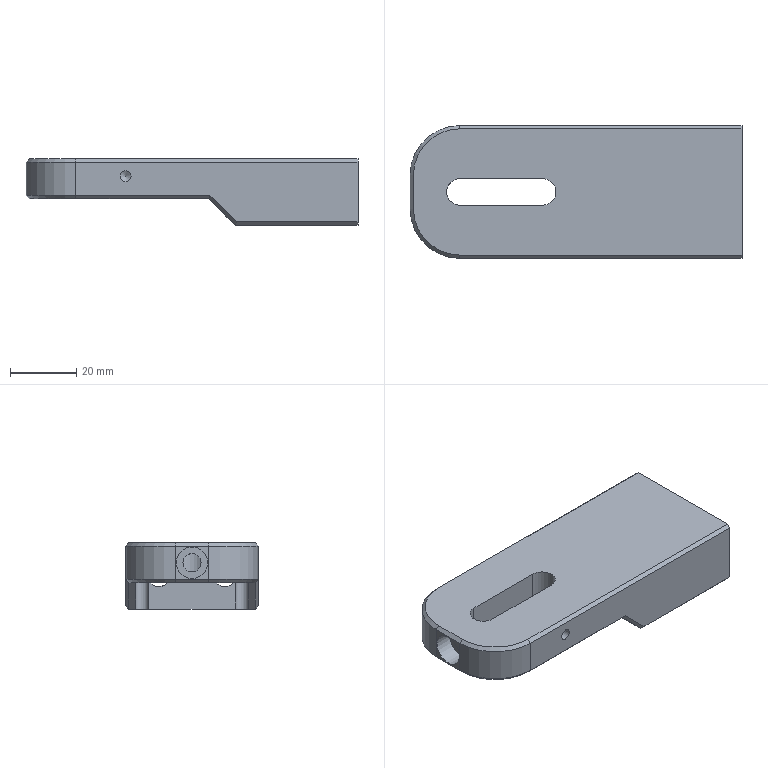Part | 1 solid | 48 faces | box 100 x 40 x 20 mm | volume 33187 mm3 | plane 28 | cylinder 14 | cone 6 | commonest cylinder face diameters 4 x4 3.3 x2 6.5 x2 8 x2 30 x2 5.5 x1
STEP:
#1=CARTESIAN_POINT('',(-37.905,2.75,-6.));
#2=VERTEX_POINT('',#1);
#3=CARTESIAN_POINT('',(-38.064,2.588,-4.884));
#4=CARTESIAN_POINT('',(-37.826,2.83,-6.002));
#5=CARTESIAN_POINT('',(-38.062,2.593,-7.11));
#6=CARTESIAN_POINT('',(-38.499,2.,-7.979));
#7=CARTESIAN_POINT('',(-38.885,1.129,-8.588));
#8=CARTESIAN_POINT('',(-39.115,-0.3754,-8.911));
#9=CARTESIAN_POINT('',(-38.65,-1.807,-8.274));
#10=CARTESIAN_POINT('',(-38.065,-2.587,-7.117));
#11=CARTESIAN_POINT('',(-37.826,-2.83,-6.007));
#12=CARTESIAN_POINT('',(-38.061,-2.591,-4.891));
#13=CARTESIAN_POINT('',(-38.645,-1.817,-3.733));
#14=CARTESIAN_POINT('',(-39.236,-0.009899,-2.929));
#15=CARTESIAN_POINT('',(-38.648,1.814,-3.73));
#16=CARTESIAN_POINT('',(-38.064,2.588,-4.884));
#17=CARTESIAN_POINT('',(-37.826,2.83,-6.002));
#18=CARTESIAN_POINT('',(-38.062,2.593,-7.11));
#19=B_SPLINE_CURVE_WITH_KNOTS('',3,(#3,#4,#5,#6,#7,#8,#9,#10,#11,#12,#13,#14,#15,#16,#17,#18),.UNSPECIFIED.,.T.,.F.,(1,1,1,1,1,1,1,1,1,1,1,1,1,1,1,1,1,1,1,1),(-0.004449,-0.002224,-0.001112,0.,0.001112,0.002224,0.003337,0.004449,0.006673,0.007786,0.008898,0.01001,0.01112,0.01335,0.01557,0.01668,0.0178,0.01891,0.02002,0.02113),.UNSPECIFIED.);
#20=EDGE_CURVE('',#2,#2,#19,.T.);
#21=ORIENTED_EDGE('',*,*,#20,.F.);
#22=EDGE_LOOP('',(#21));
#23=FACE_BOUND('',#22,.T.);
#24=CARTESIAN_POINT('',(-44.5,2.75,-6.));
#25=VERTEX_POINT('',#24);
#26=CARTESIAN_POINT('',(-44.5,0.,-6.));
#27=DIRECTION('',(1.,0.,0.));
#28=DIRECTION('',(0.,1.,0.));
#29=AXIS2_PLACEMENT_3D('',#26,#27,#28);
#30=CIRCLE('',#29,2.75);
#31=EDGE_CURVE('',#25,#25,#30,.T.);
#32=ORIENTED_EDGE('',*,*,#31,.F.);
#33=EDGE_LOOP('',(#32));
#34=FACE_BOUND('',#33,.T.);
#35=CARTESIAN_POINT('',(-35.,0.,-6.));
#36=DIRECTION('',(-1.,0.,0.));
#37=DIRECTION('',(0.,-1.,0.));
#38=AXIS2_PLACEMENT_3D('',#35,#36,#37);
#39=CYLINDRICAL_SURFACE('',#38,2.75);
#40=ADVANCED_FACE('',(#23,#34),#39,.F.);
#41=CARTESIAN_POINT('',(-50.,4.75,-6.));
#42=VERTEX_POINT('',#41);
#43=CARTESIAN_POINT('',(-50.,0.,-6.));
#44=DIRECTION('',(-1.,0.,0.));
#45=DIRECTION('',(0.,1.,0.));
#46=AXIS2_PLACEMENT_3D('',#43,#44,#45);
#47=CIRCLE('',#46,4.75);
#48=EDGE_CURVE('',#42,#42,#47,.T.);
#49=ORIENTED_EDGE('',*,*,#48,.F.);
#50=EDGE_LOOP('',(#49));
#51=FACE_BOUND('',#50,.T.);
#52=CARTESIAN_POINT('',(-50.,5.,-1.));
#53=VERTEX_POINT('',#52);
#54=CARTESIAN_POINT('',(-50.,5.,-11.));
#55=VERTEX_POINT('',#54);
#56=CARTESIAN_POINT('',(-50.,5.,-20.));
#57=DIRECTION('',(0.,0.,-1.));
#58=VECTOR('',#57,1000.);
#59=LINE('',#56,#58);
#60=EDGE_CURVE('',#53,#55,#59,.T.);
#61=ORIENTED_EDGE('',*,*,#60,.T.);
#62=CARTESIAN_POINT('',(-50.,-5.,-11.));
#63=VERTEX_POINT('',#62);
#64=CARTESIAN_POINT('',(-50.,-20.,-11.));
#65=DIRECTION('',(0.,-1.,0.));
#66=VECTOR('',#65,1000.);
#67=LINE('',#64,#66);
#68=EDGE_CURVE('',#55,#63,#67,.T.);
#69=ORIENTED_EDGE('',*,*,#68,.T.);
#70=CARTESIAN_POINT('',(-50.,-5.,-1.));
#71=VERTEX_POINT('',#70);
#72=CARTESIAN_POINT('',(-50.,-5.,-20.));
#73=DIRECTION('',(0.,0.,1.));
#74=VECTOR('',#73,1000.);
#75=LINE('',#72,#74);
#76=EDGE_CURVE('',#63,#71,#75,.T.);
#77=ORIENTED_EDGE('',*,*,#76,.T.);
#78=CARTESIAN_POINT('',(-50.,-20.,-1.));
#79=DIRECTION('',(0.,1.,0.));
#80=VECTOR('',#79,1000.);
#81=LINE('',#78,#80);
#82=EDGE_CURVE('',#71,#53,#81,.T.);
#83=ORIENTED_EDGE('',*,*,#82,.T.);
#84=EDGE_LOOP('',(#61,#69,#77,#83));
#85=FACE_BOUND('',#84,.T.);
#86=CARTESIAN_POINT('',(-50.,-20.,-20.));
#87=DIRECTION('',(1.,0.,0.));
#88=DIRECTION('',(0.,1.,0.));
#89=AXIS2_PLACEMENT_3D('',#86,#87,#88);
#90=PLANE('',#89);
#91=ADVANCED_FACE('',(#51,#85),#90,.F.);
#92=CARTESIAN_POINT('',(-18.35,20.,-5.25));
#93=VERTEX_POINT('',#92);
#94=CARTESIAN_POINT('',(-20.,20.,-5.25));
#95=DIRECTION('',(0.,1.,0.));
#96=DIRECTION('',(1.,0.,0.));
#97=AXIS2_PLACEMENT_3D('',#94,#95,#96);
#98=CIRCLE('',#97,1.65);
#99=EDGE_CURVE('',#93,#93,#98,.T.);
#100=ORIENTED_EDGE('',*,*,#99,.F.);
#101=EDGE_LOOP('',(#100));
#102=FACE_BOUND('',#101,.T.);
#103=CARTESIAN_POINT('',(50.,20.,-19.));
#104=VERTEX_POINT('',#103);
#105=CARTESIAN_POINT('',(50.,20.,-1.));
#106=VERTEX_POINT('',#105);
#107=CARTESIAN_POINT('',(50.,20.,-20.));
#108=DIRECTION('',(0.,0.,1.));
#109=VECTOR('',#108,1000.);
#110=LINE('',#107,#109);
#111=EDGE_CURVE('',#104,#106,#110,.T.);
#112=ORIENTED_EDGE('',*,*,#111,.F.);
#113=CARTESIAN_POINT('',(13.414,20.,-19.));
#114=VERTEX_POINT('',#113);
#115=CARTESIAN_POINT('',(13.,20.,-19.));
#116=DIRECTION('',(-1.,0.,0.));
#117=VECTOR('',#116,1000.);
#118=LINE('',#115,#117);
#119=EDGE_CURVE('',#104,#114,#118,.T.);
#120=ORIENTED_EDGE('',*,*,#119,.T.);
#121=CARTESIAN_POINT('',(5.414,20.,-11.));
#122=VERTEX_POINT('',#121);
#123=CARTESIAN_POINT('',(5.707,20.,-11.293));
#124=DIRECTION('',(-0.7071,0.,0.7071));
#125=VECTOR('',#124,1000.);
#126=LINE('',#123,#125);
#127=EDGE_CURVE('',#114,#122,#126,.T.);
#128=ORIENTED_EDGE('',*,*,#127,.T.);
#129=CARTESIAN_POINT('',(-35.,20.,-11.));
#130=VERTEX_POINT('',#129);
#131=CARTESIAN_POINT('',(-50.,20.,-11.));
#132=DIRECTION('',(-1.,0.,0.));
#133=VECTOR('',#132,1000.);
#134=LINE('',#131,#133);
#135=EDGE_CURVE('',#122,#130,#134,.T.);
#136=ORIENTED_EDGE('',*,*,#135,.T.);
#137=CARTESIAN_POINT('',(-35.,20.,-1.));
#138=VERTEX_POINT('',#137);
#139=CARTESIAN_POINT('',(-35.,20.,-20.));
#140=DIRECTION('',(0.,0.,1.));
#141=VECTOR('',#140,1000.);
#142=LINE('',#139,#141);
#143=EDGE_CURVE('',#130,#138,#142,.T.);
#144=ORIENTED_EDGE('',*,*,#143,.T.);
#145=CARTESIAN_POINT('',(-50.,20.,-1.));
#146=DIRECTION('',(1.,0.,0.));
#147=VECTOR('',#146,1000.);
#148=LINE('',#145,#147);
#149=EDGE_CURVE('',#138,#106,#148,.T.);
#150=ORIENTED_EDGE('',*,*,#149,.T.);
#151=EDGE_LOOP('',(#112,#120,#128,#136,#144,#150));
#152=FACE_BOUND('',#151,.T.);
#153=CARTESIAN_POINT('',(-50.,20.,-20.));
#154=DIRECTION('',(0.,-1.,0.));
#155=DIRECTION('',(1.,0.,0.));
#156=AXIS2_PLACEMENT_3D('',#153,#154,#155);
#157=PLANE('',#156);
#158=ADVANCED_FACE('',(#102,#152),#157,.F.);
#159=CARTESIAN_POINT('',(50.,13.25,-10.));
#160=VERTEX_POINT('',#159);
#161=CARTESIAN_POINT('',(50.,10.,-10.));
#162=DIRECTION('',(-1.,0.,0.));
#163=DIRECTION('',(0.,1.,0.));
#164=AXIS2_PLACEMENT_3D('',#161,#162,#163);
#165=CIRCLE('',#164,3.25);
#166=EDGE_CURVE('',#160,#160,#165,.T.);
#167=ORIENTED_EDGE('',*,*,#166,.T.);
#168=EDGE_LOOP('',(#167));
#169=FACE_BOUND('',#168,.T.);
#170=CARTESIAN_POINT('',(50.,-6.65,-10.));
#171=VERTEX_POINT('',#170);
#172=CARTESIAN_POINT('',(50.,-9.9,-10.));
#173=DIRECTION('',(-1.,0.,0.));
#174=DIRECTION('',(0.,1.,0.));
#175=AXIS2_PLACEMENT_3D('',#172,#173,#174);
#176=CIRCLE('',#175,3.25);
#177=EDGE_CURVE('',#171,#171,#176,.T.);
#178=ORIENTED_EDGE('',*,*,#177,.T.);
#179=EDGE_LOOP('',(#178));
#180=FACE_BOUND('',#179,.T.);
#181=CARTESIAN_POINT('',(50.,-20.,-19.));
#182=VERTEX_POINT('',#181);
#183=CARTESIAN_POINT('',(50.,-20.,-1.));
#184=VERTEX_POINT('',#183);
#185=CARTESIAN_POINT('',(50.,-20.,-20.));
#186=DIRECTION('',(0.,0.,1.));
#187=VECTOR('',#186,1000.);
#188=LINE('',#185,#187);
#189=EDGE_CURVE('',#182,#184,#188,.T.);
#190=ORIENTED_EDGE('',*,*,#189,.F.);
#191=CARTESIAN_POINT('',(50.,-19.,-20.));
#192=VERTEX_POINT('',#191);
#193=CARTESIAN_POINT('',(50.,-19.,-20.));
#194=DIRECTION('',(0.,0.7071,-0.7071));
#195=VECTOR('',#194,1000.);
#196=LINE('',#193,#195);
#197=EDGE_CURVE('',#182,#192,#196,.T.);
#198=ORIENTED_EDGE('',*,*,#197,.T.);
#199=CARTESIAN_POINT('',(50.,19.,-20.));
#200=VERTEX_POINT('',#199);
#201=CARTESIAN_POINT('',(50.,-20.,-20.));
#202=DIRECTION('',(0.,-1.,0.));
#203=VECTOR('',#202,1000.);
#204=LINE('',#201,#203);
#205=EDGE_CURVE('',#200,#192,#204,.T.);
#206=ORIENTED_EDGE('',*,*,#205,.F.);
#207=CARTESIAN_POINT('',(50.,19.,-20.));
#208=DIRECTION('',(0.,0.7071,0.7071));
#209=VECTOR('',#208,1000.);
#210=LINE('',#207,#209);
#211=EDGE_CURVE('',#200,#104,#210,.T.);
#212=ORIENTED_EDGE('',*,*,#211,.T.);
#213=ORIENTED_EDGE('',*,*,#111,.T.);
#214=CARTESIAN_POINT('',(50.,19.,0.));
#215=VERTEX_POINT('',#214);
#216=CARTESIAN_POINT('',(50.,20.,-1.));
#217=DIRECTION('',(0.,-0.7071,0.7071));
#218=VECTOR('',#217,1000.);
#219=LINE('',#216,#218);
#220=EDGE_CURVE('',#106,#215,#219,.T.);
#221=ORIENTED_EDGE('',*,*,#220,.T.);
#222=CARTESIAN_POINT('',(50.,-19.,0.));
#223=VERTEX_POINT('',#222);
#224=CARTESIAN_POINT('',(50.,-20.,0.));
#225=DIRECTION('',(0.,-1.,0.));
#226=VECTOR('',#225,1000.);
#227=LINE('',#224,#226);
#228=EDGE_CURVE('',#215,#223,#227,.T.);
#229=ORIENTED_EDGE('',*,*,#228,.T.);
#230=CARTESIAN_POINT('',(50.,-20.,-1.));
#231=DIRECTION('',(0.,-0.7071,-0.7071));
#232=VECTOR('',#231,1000.);
#233=LINE('',#230,#232);
#234=EDGE_CURVE('',#223,#184,#233,.T.);
#235=ORIENTED_EDGE('',*,*,#234,.T.);
#236=EDGE_LOOP('',(#190,#198,#206,#212,#213,#221,#229,#235));
#237=FACE_BOUND('',#236,.T.);
#238=CARTESIAN_POINT('',(50.,-20.,-20.));
#239=DIRECTION('',(-1.,0.,0.));
#240=DIRECTION('',(0.,-1.,0.));
#241=AXIS2_PLACEMENT_3D('',#238,#239,#240);
#242=PLANE('',#241);
#243=ADVANCED_FACE('',(#169,#180,#237),#242,.F.);
#244=CARTESIAN_POINT('',(-21.65,-20.,-5.25));
#245=VERTEX_POINT('',#244);
#246=CARTESIAN_POINT('',(-20.,-20.,-5.25));
#247=DIRECTION('',(0.,-1.,0.));
#248=DIRECTION('',(-1.,0.,0.));
#249=AXIS2_PLACEMENT_3D('',#246,#247,#248);
#250=CIRCLE('',#249,1.65);
#251=EDGE_CURVE('',#245,#245,#250,.T.);
#252=ORIENTED_EDGE('',*,*,#251,.F.);
#253=EDGE_LOOP('',(#252));
#254=FACE_BOUND('',#253,.T.);
#255=CARTESIAN_POINT('',(-35.,-20.,-1.));
#256=VERTEX_POINT('',#255);
#257=CARTESIAN_POINT('',(-35.,-20.,-11.));
#258=VERTEX_POINT('',#257);
#259=CARTESIAN_POINT('',(-35.,-20.,-20.));
#260=DIRECTION('',(0.,0.,-1.));
#261=VECTOR('',#260,1000.);
#262=LINE('',#259,#261);
#263=EDGE_CURVE('',#256,#258,#262,.T.);
#264=ORIENTED_EDGE('',*,*,#263,.T.);
#265=CARTESIAN_POINT('',(5.414,-20.,-11.));
#266=VERTEX_POINT('',#265);
#267=CARTESIAN_POINT('',(-50.,-20.,-11.));
#268=DIRECTION('',(1.,0.,0.));
#269=VECTOR('',#268,1000.);
#270=LINE('',#267,#269);
#271=EDGE_CURVE('',#258,#266,#270,.T.);
#272=ORIENTED_EDGE('',*,*,#271,.T.);
#273=CARTESIAN_POINT('',(13.414,-20.,-19.));
#274=VERTEX_POINT('',#273);
#275=CARTESIAN_POINT('',(13.707,-20.,-19.293));
#276=DIRECTION('',(0.7071,0.,-0.7071));
#277=VECTOR('',#276,1000.);
#278=LINE('',#275,#277);
#279=EDGE_CURVE('',#266,#274,#278,.T.);
#280=ORIENTED_EDGE('',*,*,#279,.T.);
#281=CARTESIAN_POINT('',(50.,-20.,-19.));
#282=DIRECTION('',(1.,0.,0.));
#283=VECTOR('',#282,1000.);
#284=LINE('',#281,#283);
#285=EDGE_CURVE('',#274,#182,#284,.T.);
#286=ORIENTED_EDGE('',*,*,#285,.T.);
#287=ORIENTED_EDGE('',*,*,#189,.T.);
#288=CARTESIAN_POINT('',(-50.,-20.,-1.));
#289=DIRECTION('',(-1.,0.,0.));
#290=VECTOR('',#289,1000.);
#291=LINE('',#288,#290);
#292=EDGE_CURVE('',#184,#256,#291,.T.);
#293=ORIENTED_EDGE('',*,*,#292,.T.);
#294=EDGE_LOOP('',(#264,#272,#280,#286,#287,#293));
#295=FACE_BOUND('',#294,.T.);
#296=CARTESIAN_POINT('',(-50.,-20.,-20.));
#297=DIRECTION('',(0.,1.,0.));
#298=DIRECTION('',(-1.,0.,0.));
#299=AXIS2_PLACEMENT_3D('',#296,#297,#298);
#300=PLANE('',#299);
#301=ADVANCED_FACE('',(#254,#295),#300,.F.);
#302=ORIENTED_EDGE('',*,*,#205,.T.);
#303=CARTESIAN_POINT('',(13.,-19.,-20.));
#304=VERTEX_POINT('',#303);
#305=CARTESIAN_POINT('',(13.,-19.,-20.));
#306=DIRECTION('',(-1.,0.,0.));
#307=VECTOR('',#306,1000.);
#308=LINE('',#305,#307);
#309=EDGE_CURVE('',#192,#304,#308,.T.);
#310=ORIENTED_EDGE('',*,*,#309,.T.);
#311=CARTESIAN_POINT('',(13.,-17.,-20.));
#312=VERTEX_POINT('',#311);
#313=CARTESIAN_POINT('',(13.,-17.,-20.));
#314=DIRECTION('',(0.,1.,0.));
#315=VECTOR('',#314,1000.);
#316=LINE('',#313,#315);
#317=EDGE_CURVE('',#304,#312,#316,.T.);
#318=ORIENTED_EDGE('',*,*,#317,.T.);
#319=CARTESIAN_POINT('',(42.,-17.,-20.));
#320=VERTEX_POINT('',#319);
#321=CARTESIAN_POINT('',(42.,-17.,-20.));
#322=DIRECTION('',(-1.,0.,0.));
#323=VECTOR('',#322,1000.);
#324=LINE('',#321,#323);
#325=EDGE_CURVE('',#320,#312,#324,.T.);
#326=ORIENTED_EDGE('',*,*,#325,.F.);
#327=CARTESIAN_POINT('',(42.,-13.,-20.));
#328=VERTEX_POINT('',#327);
#329=CARTESIAN_POINT('',(42.,-15.,-20.));
#330=DIRECTION('',(0.,0.,-1.));
#331=DIRECTION('',(0.,1.,0.));
#332=AXIS2_PLACEMENT_3D('',#329,#330,#331);
#333=CIRCLE('',#332,2.);
#334=EDGE_CURVE('',#328,#320,#333,.T.);
#335=ORIENTED_EDGE('',*,*,#334,.F.);
#336=CARTESIAN_POINT('',(42.,13.,-20.));
#337=VERTEX_POINT('',#336);
#338=CARTESIAN_POINT('',(42.,-17.,-20.));
#339=DIRECTION('',(0.,-1.,0.));
#340=VECTOR('',#339,1000.);
#341=LINE('',#338,#340);
#342=EDGE_CURVE('',#337,#328,#341,.T.);
#343=ORIENTED_EDGE('',*,*,#342,.F.);
#344=CARTESIAN_POINT('',(42.,17.,-20.));
#345=VERTEX_POINT('',#344);
#346=CARTESIAN_POINT('',(42.,15.,-20.));
#347=DIRECTION('',(0.,0.,-1.));
#348=DIRECTION('',(0.,1.,0.));
#349=AXIS2_PLACEMENT_3D('',#346,#347,#348);
#350=CIRCLE('',#349,2.);
#351=EDGE_CURVE('',#345,#337,#350,.T.);
#352=ORIENTED_EDGE('',*,*,#351,.F.);
#353=CARTESIAN_POINT('',(13.,17.,-20.));
#354=VERTEX_POINT('',#353);
#355=CARTESIAN_POINT('',(42.,17.,-20.));
#356=DIRECTION('',(1.,0.,0.));
#357=VECTOR('',#356,1000.);
#358=LINE('',#355,#357);
#359=EDGE_CURVE('',#354,#345,#358,.T.);
#360=ORIENTED_EDGE('',*,*,#359,.F.);
#361=CARTESIAN_POINT('',(13.,19.,-20.));
#362=VERTEX_POINT('',#361);
#363=CARTESIAN_POINT('',(13.,20.,-20.));
#364=DIRECTION('',(0.,1.,0.));
#365=VECTOR('',#364,1000.);
#366=LINE('',#363,#365);
#367=EDGE_CURVE('',#354,#362,#366,.T.);
#368=ORIENTED_EDGE('',*,*,#367,.T.);
#369=CARTESIAN_POINT('',(50.,19.,-20.));
#370=DIRECTION('',(1.,0.,0.));
#371=VECTOR('',#370,1000.);
#372=LINE('',#369,#371);
#373=EDGE_CURVE('',#362,#200,#372,.T.);
#374=ORIENTED_EDGE('',*,*,#373,.T.);
#375=EDGE_LOOP('',(#302,#310,#318,#326,#335,#343,#352,#360,#368,#374));
#376=FACE_BOUND('',#375,.T.);
#377=CARTESIAN_POINT('',(-50.,20.,-20.));
#378=DIRECTION('',(0.,0.,-1.));
#379=DIRECTION('',(0.,-1.,0.));
#380=AXIS2_PLACEMENT_3D('',#377,#378,#379);
#381=PLANE('',#380);
#382=ADVANCED_FACE('',(#376),#381,.T.);
#383=CARTESIAN_POINT('',(-10.,4.,0.));
#384=VERTEX_POINT('',#383);
#385=CARTESIAN_POINT('',(-35.,4.,0.));
#386=VERTEX_POINT('',#385);
#387=CARTESIAN_POINT('',(-10.,4.,0.));
#388=DIRECTION('',(-1.,0.,0.));
#389=VECTOR('',#388,1000.);
#390=LINE('',#387,#389);
#391=EDGE_CURVE('',#384,#386,#390,.T.);
#392=ORIENTED_EDGE('',*,*,#391,.F.);
#393=CARTESIAN_POINT('',(-10.,-4.,0.));
#394=VERTEX_POINT('',#393);
#395=CARTESIAN_POINT('',(-10.,0.,0.));
#396=DIRECTION('',(0.,0.,1.));
#397=DIRECTION('',(0.,-1.,0.));
#398=AXIS2_PLACEMENT_3D('',#395,#396,#397);
#399=CIRCLE('',#398,4.);
#400=EDGE_CURVE('',#394,#384,#399,.T.);
#401=ORIENTED_EDGE('',*,*,#400,.F.);
#402=CARTESIAN_POINT('',(-35.,-4.,0.));
#403=VERTEX_POINT('',#402);
#404=CARTESIAN_POINT('',(-10.,-4.,0.));
#405=DIRECTION('',(1.,0.,0.));
#406=VECTOR('',#405,1000.);
#407=LINE('',#404,#406);
#408=EDGE_CURVE('',#403,#394,#407,.T.);
#409=ORIENTED_EDGE('',*,*,#408,.F.);
#410=CARTESIAN_POINT('',(-35.,0.,0.));
#411=DIRECTION('',(0.,0.,1.));
#412=DIRECTION('',(0.,-1.,0.));
#413=AXIS2_PLACEMENT_3D('',#410,#411,#412);
#414=CIRCLE('',#413,4.);
#415=EDGE_CURVE('',#386,#403,#414,.T.);
#416=ORIENTED_EDGE('',*,*,#415,.F.);
#417=EDGE_LOOP('',(#392,#401,#409,#416));
#418=FACE_BOUND('',#417,.T.);
#419=CARTESIAN_POINT('',(-49.,-5.,0.));
#420=VERTEX_POINT('',#419);
#421=CARTESIAN_POINT('',(-35.,-19.,0.));
#422=VERTEX_POINT('',#421);
#423=CARTESIAN_POINT('',(-35.,-5.,0.));
#424=DIRECTION('',(0.,0.,1.));
#425=DIRECTION('',(0.,1.,0.));
#426=AXIS2_PLACEMENT_3D('',#423,#424,#425);
#427=CIRCLE('',#426,14.);
#428=EDGE_CURVE('',#420,#422,#427,.T.);
#429=ORIENTED_EDGE('',*,*,#428,.T.);
#430=CARTESIAN_POINT('',(-50.,-19.,0.));
#431=DIRECTION('',(1.,0.,0.));
#432=VECTOR('',#431,1000.);
#433=LINE('',#430,#432);
#434=EDGE_CURVE('',#422,#223,#433,.T.);
#435=ORIENTED_EDGE('',*,*,#434,.T.);
#436=ORIENTED_EDGE('',*,*,#228,.F.);
#437=CARTESIAN_POINT('',(-35.,19.,0.));
#438=VERTEX_POINT('',#437);
#439=CARTESIAN_POINT('',(-50.,19.,0.));
#440=DIRECTION('',(-1.,0.,0.));
#441=VECTOR('',#440,1000.);
#442=LINE('',#439,#441);
#443=EDGE_CURVE('',#215,#438,#442,.T.);
#444=ORIENTED_EDGE('',*,*,#443,.T.);
#445=CARTESIAN_POINT('',(-49.,5.,0.));
#446=VERTEX_POINT('',#445);
#447=CARTESIAN_POINT('',(-35.,5.,0.));
#448=DIRECTION('',(0.,0.,1.));
#449=DIRECTION('',(0.,1.,0.));
#450=AXIS2_PLACEMENT_3D('',#447,#448,#449);
#451=CIRCLE('',#450,14.);
#452=EDGE_CURVE('',#438,#446,#451,.T.);
#453=ORIENTED_EDGE('',*,*,#452,.T.);
#454=CARTESIAN_POINT('',(-49.,20.,0.));
#455=DIRECTION('',(0.,-1.,0.));
#456=VECTOR('',#455,1000.);
#457=LINE('',#454,#456);
#458=EDGE_CURVE('',#446,#420,#457,.T.);
#459=ORIENTED_EDGE('',*,*,#458,.T.);
#460=EDGE_LOOP('',(#429,#435,#436,#444,#453,#459));
#461=FACE_BOUND('',#460,.T.);
#462=CARTESIAN_POINT('',(-50.,20.,0.));
#463=DIRECTION('',(0.,0.,-1.));
#464=DIRECTION('',(0.,-1.,0.));
#465=AXIS2_PLACEMENT_3D('',#462,#463,#464);
#466=PLANE('',#465);
#467=ADVANCED_FACE('',(#418,#461),#466,.F.);
#468=CARTESIAN_POINT('',(42.,13.,-3.));
#469=VERTEX_POINT('',#468);
#470=CARTESIAN_POINT('',(42.,13.,-8.75));
#471=VERTEX_POINT('',#470);
#472=CARTESIAN_POINT('',(42.,13.,2.657));
#473=DIRECTION('',(0.,0.,-1.));
#474=VECTOR('',#473,1000.);
#475=LINE('',#472,#474);
#476=EDGE_CURVE('',#469,#471,#475,.T.);
#477=ORIENTED_EDGE('',*,*,#476,.T.);
#478=CARTESIAN_POINT('',(42.,13.,-11.25));
#479=VERTEX_POINT('',#478);
#480=CARTESIAN_POINT('',(42.,10.,-10.));
#481=DIRECTION('',(-1.,0.,0.));
#482=DIRECTION('',(0.,1.,0.));
#483=AXIS2_PLACEMENT_3D('',#480,#481,#482);
#484=CIRCLE('',#483,3.25);
#485=EDGE_CURVE('',#479,#471,#484,.T.);
#486=ORIENTED_EDGE('',*,*,#485,.F.);
#487=CARTESIAN_POINT('',(42.,13.,2.657));
#488=DIRECTION('',(0.,0.,-1.));
#489=VECTOR('',#488,1000.);
#490=LINE('',#487,#489);
#491=EDGE_CURVE('',#479,#337,#490,.T.);
#492=ORIENTED_EDGE('',*,*,#491,.T.);
#493=ORIENTED_EDGE('',*,*,#342,.T.);
#494=CARTESIAN_POINT('',(42.,-13.,-10.976));
#495=VERTEX_POINT('',#494);
#496=CARTESIAN_POINT('',(42.,-13.,2.657));
#497=DIRECTION('',(0.,0.,1.));
#498=VECTOR('',#497,1000.);
#499=LINE('',#496,#498);
#500=EDGE_CURVE('',#328,#495,#499,.T.);
#501=ORIENTED_EDGE('',*,*,#500,.T.);
#502=CARTESIAN_POINT('',(42.,-13.,-9.024));
#503=VERTEX_POINT('',#502);
#504=CARTESIAN_POINT('',(42.,-9.9,-10.));
#505=DIRECTION('',(-1.,0.,0.));
#506=DIRECTION('',(0.,1.,0.));
#507=AXIS2_PLACEMENT_3D('',#504,#505,#506);
#508=CIRCLE('',#507,3.25);
#509=EDGE_CURVE('',#503,#495,#508,.T.);
#510=ORIENTED_EDGE('',*,*,#509,.F.);
#511=CARTESIAN_POINT('',(42.,-13.,-3.));
#512=VERTEX_POINT('',#511);
#513=CARTESIAN_POINT('',(42.,-13.,2.657));
#514=DIRECTION('',(0.,0.,1.));
#515=VECTOR('',#514,1000.);
#516=LINE('',#513,#515);
#517=EDGE_CURVE('',#503,#512,#516,.T.);
#518=ORIENTED_EDGE('',*,*,#517,.T.);
#519=CARTESIAN_POINT('',(42.,-17.,-3.));
#520=DIRECTION('',(0.,-1.,0.));
#521=VECTOR('',#520,1000.);
#522=LINE('',#519,#521);
#523=EDGE_CURVE('',#469,#512,#522,.T.);
#524=ORIENTED_EDGE('',*,*,#523,.F.);
#525=EDGE_LOOP('',(#477,#486,#492,#493,#501,#510,#518,#524));
#526=FACE_BOUND('',#525,.T.);
#527=CARTESIAN_POINT('',(42.,-17.,-3.));
#528=DIRECTION('',(1.,0.,0.));
#529=DIRECTION('',(0.,1.,0.));
#530=AXIS2_PLACEMENT_3D('',#527,#528,#529);
#531=PLANE('',#530);
#532=ADVANCED_FACE('',(#526),#531,.F.);
#533=CARTESIAN_POINT('',(2.,17.,-3.));
#534=VERTEX_POINT('',#533);
#535=CARTESIAN_POINT('',(42.,17.,-3.));
#536=VERTEX_POINT('',#535);
#537=CARTESIAN_POINT('',(42.,17.,-3.));
#538=DIRECTION('',(1.,0.,0.));
#539=VECTOR('',#538,1000.);
#540=LINE('',#537,#539);
#541=EDGE_CURVE('',#534,#536,#540,.T.);
#542=ORIENTED_EDGE('',*,*,#541,.F.);
#543=CARTESIAN_POINT('',(2.,17.,-6.));
#544=VERTEX_POINT('',#543);
#545=CARTESIAN_POINT('',(2.,17.,-8.));
#546=DIRECTION('',(0.,0.,-1.));
#547=VECTOR('',#546,1000.);
#548=LINE('',#545,#547);
#549=EDGE_CURVE('',#534,#544,#548,.T.);
#550=ORIENTED_EDGE('',*,*,#549,.T.);
#551=CARTESIAN_POINT('',(-4.,17.,-12.));
#552=VERTEX_POINT('',#551);
#553=CARTESIAN_POINT('',(23.5,17.,15.5));
#554=DIRECTION('',(-0.7071,0.,-0.7071));
#555=VECTOR('',#554,1000.);
#556=LINE('',#553,#555);
#557=EDGE_CURVE('',#544,#552,#556,.T.);
#558=ORIENTED_EDGE('',*,*,#557,.T.);
#559=CARTESIAN_POINT('',(5.,17.,-12.));
#560=VERTEX_POINT('',#559);
#561=CARTESIAN_POINT('',(42.,17.,-12.));
#562=DIRECTION('',(1.,0.,0.));
#563=VECTOR('',#562,1000.);
#564=LINE('',#561,#563);
#565=EDGE_CURVE('',#552,#560,#564,.T.);
#566=ORIENTED_EDGE('',*,*,#565,.T.);
#567=CARTESIAN_POINT('',(5.,17.,-12.));
#568=DIRECTION('',(0.7071,0.,-0.7071));
#569=VECTOR('',#568,1000.);
#570=LINE('',#567,#569);
#571=EDGE_CURVE('',#560,#354,#570,.T.);
#572=ORIENTED_EDGE('',*,*,#571,.T.);
#573=ORIENTED_EDGE('',*,*,#359,.T.);
#574=CARTESIAN_POINT('',(42.,17.,-3.));
#575=DIRECTION('',(0.,0.,-1.));
#576=VECTOR('',#575,1000.);
#577=LINE('',#574,#576);
#578=EDGE_CURVE('',#536,#345,#577,.T.);
#579=ORIENTED_EDGE('',*,*,#578,.F.);
#580=EDGE_LOOP('',(#542,#550,#558,#566,#572,#573,#579));
#581=FACE_BOUND('',#580,.T.);
#582=CARTESIAN_POINT('',(42.,17.,-3.));
#583=DIRECTION('',(0.,1.,0.));
#584=DIRECTION('',(-1.,0.,0.));
#585=AXIS2_PLACEMENT_3D('',#582,#583,#584);
#586=PLANE('',#585);
#587=ADVANCED_FACE('',(#581),#586,.F.);
#588=CARTESIAN_POINT('',(0.,-15.,-8.));
#589=VERTEX_POINT('',#588);
#590=CARTESIAN_POINT('',(0.,15.,-8.));
#591=VERTEX_POINT('',#590);
#592=CARTESIAN_POINT('',(0.,-17.,-8.));
#593=DIRECTION('',(0.,1.,0.));
#594=VECTOR('',#593,1000.);
#595=LINE('',#592,#594);
#596=EDGE_CURVE('',#589,#591,#595,.T.);
#597=ORIENTED_EDGE('',*,*,#596,.T.);
#598=CARTESIAN_POINT('',(0.,15.,-3.));
#599=VERTEX_POINT('',#598);
#600=CARTESIAN_POINT('',(0.,15.,-3.));
#601=DIRECTION('',(0.,0.,1.));
#602=VECTOR('',#601,1000.);
#603=LINE('',#600,#602);
#604=EDGE_CURVE('',#591,#599,#603,.T.);
#605=ORIENTED_EDGE('',*,*,#604,.T.);
#606=CARTESIAN_POINT('',(0.,-15.,-3.));
#607=VERTEX_POINT('',#606);
#608=CARTESIAN_POINT('',(0.,-17.,-3.));
#609=DIRECTION('',(0.,1.,0.));
#610=VECTOR('',#609,1000.);
#611=LINE('',#608,#610);
#612=EDGE_CURVE('',#607,#599,#611,.T.);
#613=ORIENTED_EDGE('',*,*,#612,.F.);
#614=CARTESIAN_POINT('',(0.,-15.,-8.));
#615=DIRECTION('',(0.,0.,-1.));
#616=VECTOR('',#615,1000.);
#617=LINE('',#614,#616);
#618=EDGE_CURVE('',#607,#589,#617,.T.);
#619=ORIENTED_EDGE('',*,*,#618,.T.);
#620=EDGE_LOOP('',(#597,#605,#613,#619));
#621=FACE_BOUND('',#620,.T.);
#622=CARTESIAN_POINT('',(0.,-17.,-3.));
#623=DIRECTION('',(-1.,0.,0.));
#624=DIRECTION('',(0.,-1.,0.));
#625=AXIS2_PLACEMENT_3D('',#622,#623,#624);
#626=PLANE('',#625);
#627=ADVANCED_FACE('',(#621),#626,.F.);
#628=CARTESIAN_POINT('',(-4.,-17.,-12.));
#629=VERTEX_POINT('',#628);
#630=CARTESIAN_POINT('',(2.,-17.,-6.));
#631=VERTEX_POINT('',#630);
#632=CARTESIAN_POINT('',(23.5,-17.,15.5));
#633=DIRECTION('',(0.7071,0.,0.7071));
#634=VECTOR('',#633,1000.);
#635=LINE('',#632,#634);
#636=EDGE_CURVE('',#629,#631,#635,.T.);
#637=ORIENTED_EDGE('',*,*,#636,.T.);
#638=CARTESIAN_POINT('',(2.,-17.,-3.));
#639=VERTEX_POINT('',#638);
#640=CARTESIAN_POINT('',(2.,-17.,-3.));
#641=DIRECTION('',(0.,0.,1.));
#642=VECTOR('',#641,1000.);
#643=LINE('',#640,#642);
#644=EDGE_CURVE('',#631,#639,#643,.T.);
#645=ORIENTED_EDGE('',*,*,#644,.T.);
#646=CARTESIAN_POINT('',(42.,-17.,-3.));
#647=VERTEX_POINT('',#646);
#648=CARTESIAN_POINT('',(42.,-17.,-3.));
#649=DIRECTION('',(-1.,0.,0.));
#650=VECTOR('',#649,1000.);
#651=LINE('',#648,#650);
#652=EDGE_CURVE('',#647,#639,#651,.T.);
#653=ORIENTED_EDGE('',*,*,#652,.F.);
#654=CARTESIAN_POINT('',(42.,-17.,-3.));
#655=DIRECTION('',(0.,0.,-1.));
#656=VECTOR('',#655,1000.);
#657=LINE('',#654,#656);
#658=EDGE_CURVE('',#647,#320,#657,.T.);
#659=ORIENTED_EDGE('',*,*,#658,.T.);
#660=ORIENTED_EDGE('',*,*,#325,.T.);
#661=CARTESIAN_POINT('',(5.,-17.,-12.));
#662=VERTEX_POINT('',#661);
#663=CARTESIAN_POINT('',(5.,-17.,-12.));
#664=DIRECTION('',(-0.7071,0.,0.7071));
#665=VECTOR('',#664,1000.);
#666=LINE('',#663,#665);
#667=EDGE_CURVE('',#312,#662,#666,.T.);
#668=ORIENTED_EDGE('',*,*,#667,.T.);
#669=CARTESIAN_POINT('',(42.,-17.,-12.));
#670=DIRECTION('',(-1.,0.,0.));
#671=VECTOR('',#670,1000.);
#672=LINE('',#669,#671);
#673=EDGE_CURVE('',#662,#629,#672,.T.);
#674=ORIENTED_EDGE('',*,*,#673,.T.);
#675=EDGE_LOOP('',(#637,#645,#653,#659,#660,#668,#674));
#676=FACE_BOUND('',#675,.T.);
#677=CARTESIAN_POINT('',(42.,-17.,-3.));
#678=DIRECTION('',(0.,-1.,0.));
#679=DIRECTION('',(1.,0.,0.));
#680=AXIS2_PLACEMENT_3D('',#677,#678,#679);
#681=PLANE('',#680);
#682=ADVANCED_FACE('',(#676),#681,.F.);
#683=ORIENTED_EDGE('',*,*,#612,.T.);
#684=CARTESIAN_POINT('',(2.,15.,-3.));
#685=DIRECTION('',(0.,0.,-1.));
#686=DIRECTION('',(0.,-1.,0.));
#687=AXIS2_PLACEMENT_3D('',#684,#685,#686);
#688=CIRCLE('',#687,2.);
#689=EDGE_CURVE('',#599,#534,#688,.T.);
#690=ORIENTED_EDGE('',*,*,#689,.T.);
#691=ORIENTED_EDGE('',*,*,#541,.T.);
#692=CARTESIAN_POINT('',(42.,15.,-3.));
#693=DIRECTION('',(0.,0.,-1.));
#694=DIRECTION('',(0.,-1.,0.));
#695=AXIS2_PLACEMENT_3D('',#692,#693,#694);
#696=CIRCLE('',#695,2.);
#697=EDGE_CURVE('',#536,#469,#696,.T.);
#698=ORIENTED_EDGE('',*,*,#697,.T.);
#699=ORIENTED_EDGE('',*,*,#523,.T.);
#700=CARTESIAN_POINT('',(42.,-15.,-3.));
#701=DIRECTION('',(0.,0.,-1.));
#702=DIRECTION('',(0.,-1.,0.));
#703=AXIS2_PLACEMENT_3D('',#700,#701,#702);
#704=CIRCLE('',#703,2.);
#705=EDGE_CURVE('',#512,#647,#704,.T.);
#706=ORIENTED_EDGE('',*,*,#705,.T.);
#707=ORIENTED_EDGE('',*,*,#652,.T.);
#708=CARTESIAN_POINT('',(2.,-15.,-3.));
#709=DIRECTION('',(0.,0.,-1.));
#710=DIRECTION('',(0.,-1.,0.));
#711=AXIS2_PLACEMENT_3D('',#708,#709,#710);
#712=CIRCLE('',#711,2.);
#713=EDGE_CURVE('',#639,#607,#712,.T.);
#714=ORIENTED_EDGE('',*,*,#713,.T.);
#715=EDGE_LOOP('',(#683,#690,#691,#698,#699,#706,#707,#714));
#716=FACE_BOUND('',#715,.T.);
#717=CARTESIAN_POINT('',(0.,0.,-3.));
#718=DIRECTION('',(0.,0.,1.));
#719=DIRECTION('',(0.,1.,0.));
#720=AXIS2_PLACEMENT_3D('',#717,#718,#719);
#721=PLANE('',#720);
#722=ADVANCED_FACE('',(#716),#721,.F.);
#723=CARTESIAN_POINT('',(-35.,-4.,-12.));
#724=VERTEX_POINT('',#723);
#725=CARTESIAN_POINT('',(-10.,-4.,-12.));
#726=VERTEX_POINT('',#725);
#727=CARTESIAN_POINT('',(-50.,-4.,-12.));
#728=DIRECTION('',(1.,0.,0.));
#729=VECTOR('',#728,1000.);
#730=LINE('',#727,#729);
#731=EDGE_CURVE('',#724,#726,#730,.T.);
#732=ORIENTED_EDGE('',*,*,#731,.T.);
#733=CARTESIAN_POINT('',(-10.,4.,-12.));
#734=VERTEX_POINT('',#733);
#735=CARTESIAN_POINT('',(-10.,0.,-12.));
#736=DIRECTION('',(0.,0.,1.));
#737=DIRECTION('',(1.,0.,0.));
#738=AXIS2_PLACEMENT_3D('',#735,#736,#737);
#739=CIRCLE('',#738,4.);
#740=EDGE_CURVE('',#726,#734,#739,.T.);
#741=ORIENTED_EDGE('',*,*,#740,.T.);
#742=CARTESIAN_POINT('',(-35.,4.,-12.));
#743=VERTEX_POINT('',#742);
#744=CARTESIAN_POINT('',(-50.,4.,-12.));
#745=DIRECTION('',(-1.,0.,0.));
#746=VECTOR('',#745,1000.);
#747=LINE('',#744,#746);
#748=EDGE_CURVE('',#734,#743,#747,.T.);
#749=ORIENTED_EDGE('',*,*,#748,.T.);
#750=CARTESIAN_POINT('',(-35.,0.,-12.));
#751=DIRECTION('',(0.,0.,1.));
#752=DIRECTION('',(1.,0.,0.));
#753=AXIS2_PLACEMENT_3D('',#750,#751,#752);
#754=CIRCLE('',#753,4.);
#755=EDGE_CURVE('',#743,#724,#754,.T.);
#756=ORIENTED_EDGE('',*,*,#755,.T.);
#757=EDGE_LOOP('',(#732,#741,#749,#756));
#758=FACE_BOUND('',#757,.T.);
#759=CARTESIAN_POINT('',(5.,-19.,-12.));
#760=VERTEX_POINT('',#759);
#761=CARTESIAN_POINT('',(5.,20.,-12.));
#762=DIRECTION('',(0.,-1.,0.));
#763=VECTOR('',#762,1000.);
#764=LINE('',#761,#763);
#765=EDGE_CURVE('',#662,#760,#764,.T.);
#766=ORIENTED_EDGE('',*,*,#765,.T.);
#767=CARTESIAN_POINT('',(-35.,-19.,-12.));
#768=VERTEX_POINT('',#767);
#769=CARTESIAN_POINT('',(-50.,-19.,-12.));
#770=DIRECTION('',(-1.,0.,0.));
#771=VECTOR('',#770,1000.);
#772=LINE('',#769,#771);
#773=EDGE_CURVE('',#760,#768,#772,.T.);
#774=ORIENTED_EDGE('',*,*,#773,.T.);
#775=CARTESIAN_POINT('',(-49.,-5.,-12.));
#776=VERTEX_POINT('',#775);
#777=CARTESIAN_POINT('',(-35.,-5.,-12.));
#778=DIRECTION('',(0.,0.,-1.));
#779=DIRECTION('',(1.,0.,0.));
#780=AXIS2_PLACEMENT_3D('',#777,#778,#779);
#781=CIRCLE('',#780,14.);
#782=EDGE_CURVE('',#768,#776,#781,.T.);
#783=ORIENTED_EDGE('',*,*,#782,.T.);
#784=CARTESIAN_POINT('',(-49.,5.,-12.));
#785=VERTEX_POINT('',#784);
#786=CARTESIAN_POINT('',(-49.,20.,-12.));
#787=DIRECTION('',(0.,1.,0.));
#788=VECTOR('',#787,1000.);
#789=LINE('',#786,#788);
#790=EDGE_CURVE('',#776,#785,#789,.T.);
#791=ORIENTED_EDGE('',*,*,#790,.T.);
#792=CARTESIAN_POINT('',(-35.,19.,-12.));
#793=VERTEX_POINT('',#792);
#794=CARTESIAN_POINT('',(-35.,5.,-12.));
#795=DIRECTION('',(0.,0.,-1.));
#796=DIRECTION('',(1.,0.,0.));
#797=AXIS2_PLACEMENT_3D('',#794,#795,#796);
#798=CIRCLE('',#797,14.);
#799=EDGE_CURVE('',#785,#793,#798,.T.);
#800=ORIENTED_EDGE('',*,*,#799,.T.);
#801=CARTESIAN_POINT('',(5.,19.,-12.));
#802=VERTEX_POINT('',#801);
#803=CARTESIAN_POINT('',(-50.,19.,-12.));
#804=DIRECTION('',(1.,0.,0.));
#805=VECTOR('',#804,1000.);
#806=LINE('',#803,#805);
#807=EDGE_CURVE('',#793,#802,#806,.T.);
#808=ORIENTED_EDGE('',*,*,#807,.T.);
#809=CARTESIAN_POINT('',(5.,20.,-12.));
#810=DIRECTION('',(0.,-1.,0.));
#811=VECTOR('',#810,1000.);
#812=LINE('',#809,#811);
#813=EDGE_CURVE('',#802,#560,#812,.T.);
#814=ORIENTED_EDGE('',*,*,#813,.T.);
#815=ORIENTED_EDGE('',*,*,#565,.F.);
#816=CARTESIAN_POINT('',(-4.,20.,-12.));
#817=DIRECTION('',(0.,-1.,0.));
#818=VECTOR('',#817,1000.);
#819=LINE('',#816,#818);
#820=EDGE_CURVE('',#552,#629,#819,.T.);
#821=ORIENTED_EDGE('',*,*,#820,.T.);
#822=ORIENTED_EDGE('',*,*,#673,.F.);
#823=EDGE_LOOP('',(#766,#774,#783,#791,#800,#808,#814,#815,#821,#822));
#824=FACE_BOUND('',#823,.T.);
#825=CARTESIAN_POINT('',(-50.,20.,-12.));
#826=DIRECTION('',(0.,0.,1.));
#827=DIRECTION('',(-1.,0.,0.));
#828=AXIS2_PLACEMENT_3D('',#825,#826,#827);
#829=PLANE('',#828);
#830=ADVANCED_FACE('',(#758,#824),#829,.F.);
#831=ORIENTED_EDGE('',*,*,#517,.F.);
#832=CARTESIAN_POINT('',(42.,-13.,-9.024));
#833=CARTESIAN_POINT('',(42.233,-13.,-9.024));
#834=CARTESIAN_POINT('',(42.651,-13.093,-9.302));
#835=CARTESIAN_POINT('',(42.814,-13.178,-10.001));
#836=CARTESIAN_POINT('',(42.652,-13.094,-10.696));
#837=CARTESIAN_POINT('',(42.234,-13.,-10.976));
#838=CARTESIAN_POINT('',(42.,-13.,-10.976));
#839=B_SPLINE_CURVE_WITH_KNOTS('',3,(#832,#833,#834,#835,#836,#837,#838),.UNSPECIFIED.,.F.,.F.,(4,1,1,1,4),(0.,0.0006882,0.001376,0.002065,0.002753),.UNSPECIFIED.);
#840=EDGE_CURVE('',#503,#495,#839,.T.);
#841=ORIENTED_EDGE('',*,*,#840,.T.);
#842=ORIENTED_EDGE('',*,*,#500,.F.);
#843=ORIENTED_EDGE('',*,*,#334,.T.);
#844=ORIENTED_EDGE('',*,*,#658,.F.);
#845=ORIENTED_EDGE('',*,*,#705,.F.);
#846=EDGE_LOOP('',(#831,#841,#842,#843,#844,#845));
#847=FACE_BOUND('',#846,.T.);
#848=CARTESIAN_POINT('',(42.,-15.,2.657));
#849=DIRECTION('',(0.,0.,-1.));
#850=DIRECTION('',(0.,-1.,0.));
#851=AXIS2_PLACEMENT_3D('',#848,#849,#850);
#852=CYLINDRICAL_SURFACE('',#851,2.);
#853=ADVANCED_FACE('',(#847),#852,.F.);
#854=ORIENTED_EDGE('',*,*,#491,.F.);
#855=CARTESIAN_POINT('',(42.,13.,-11.25));
#856=CARTESIAN_POINT('',(42.301,13.,-11.25));
#857=CARTESIAN_POINT('',(42.838,13.156,-10.899));
#858=CARTESIAN_POINT('',(43.034,13.297,-9.998));
#859=CARTESIAN_POINT('',(42.837,13.155,-9.1));
#860=CARTESIAN_POINT('',(42.301,13.,-8.75));
#861=CARTESIAN_POINT('',(42.,13.,-8.75));
#862=B_SPLINE_CURVE_WITH_KNOTS('',3,(#855,#856,#857,#858,#859,#860,#861),.UNSPECIFIED.,.F.,.F.,(4,1,1,1,4),(0.,0.0008877,0.001775,0.002663,0.003551),.UNSPECIFIED.);
#863=EDGE_CURVE('',#479,#471,#862,.T.);
#864=ORIENTED_EDGE('',*,*,#863,.T.);
#865=ORIENTED_EDGE('',*,*,#476,.F.);
#866=ORIENTED_EDGE('',*,*,#697,.F.);
#867=ORIENTED_EDGE('',*,*,#578,.T.);
#868=ORIENTED_EDGE('',*,*,#351,.T.);
#869=EDGE_LOOP('',(#854,#864,#865,#866,#867,#868));
#870=FACE_BOUND('',#869,.T.);
#871=CARTESIAN_POINT('',(42.,15.,2.657));
#872=DIRECTION('',(0.,0.,-1.));
#873=DIRECTION('',(0.,-1.,0.));
#874=AXIS2_PLACEMENT_3D('',#871,#872,#873);
#875=CYLINDRICAL_SURFACE('',#874,2.);
#876=ADVANCED_FACE('',(#870),#875,.F.);
#877=ORIENTED_EDGE('',*,*,#813,.F.);
#878=CARTESIAN_POINT('',(13.,19.,-20.));
#879=DIRECTION('',(0.7071,0.,-0.7071));
#880=VECTOR('',#879,1000.);
#881=LINE('',#878,#880);
#882=EDGE_CURVE('',#802,#362,#881,.T.);
#883=ORIENTED_EDGE('',*,*,#882,.T.);
#884=ORIENTED_EDGE('',*,*,#367,.F.);
#885=ORIENTED_EDGE('',*,*,#571,.F.);
#886=EDGE_LOOP('',(#877,#883,#884,#885));
#887=FACE_BOUND('',#886,.T.);
#888=CARTESIAN_POINT('',(5.,20.,-12.));
#889=DIRECTION('',(-0.7071,0.,-0.7071));
#890=DIRECTION('',(0.,-1.,0.));
#891=AXIS2_PLACEMENT_3D('',#888,#889,#890);
#892=PLANE('',#891);
#893=ADVANCED_FACE('',(#887),#892,.T.);
#894=ORIENTED_EDGE('',*,*,#317,.F.);
#895=CARTESIAN_POINT('',(5.,-19.,-12.));
#896=DIRECTION('',(-0.7071,0.,0.7071));
#897=VECTOR('',#896,1000.);
#898=LINE('',#895,#897);
#899=EDGE_CURVE('',#304,#760,#898,.T.);
#900=ORIENTED_EDGE('',*,*,#899,.T.);
#901=ORIENTED_EDGE('',*,*,#765,.F.);
#902=ORIENTED_EDGE('',*,*,#667,.F.);
#903=EDGE_LOOP('',(#894,#900,#901,#902));
#904=FACE_BOUND('',#903,.T.);
#905=CARTESIAN_POINT('',(5.,20.,-12.));
#906=DIRECTION('',(-0.7071,0.,-0.7071));
#907=DIRECTION('',(0.,-1.,0.));
#908=AXIS2_PLACEMENT_3D('',#905,#906,#907);
#909=PLANE('',#908);
#910=ADVANCED_FACE('',(#904),#909,.T.);
#911=ORIENTED_EDGE('',*,*,#143,.F.);
#912=CARTESIAN_POINT('',(-35.,5.,-11.));
#913=DIRECTION('',(0.,0.,1.));
#914=DIRECTION('',(0.,-1.,0.));
#915=AXIS2_PLACEMENT_3D('',#912,#913,#914);
#916=CIRCLE('',#915,15.);
#917=EDGE_CURVE('',#130,#55,#916,.T.);
#918=ORIENTED_EDGE('',*,*,#917,.T.);
#919=ORIENTED_EDGE('',*,*,#60,.F.);
#920=CARTESIAN_POINT('',(-35.,5.,-1.));
#921=DIRECTION('',(0.,0.,-1.));
#922=DIRECTION('',(0.,1.,0.));
#923=AXIS2_PLACEMENT_3D('',#920,#921,#922);
#924=CIRCLE('',#923,15.);
#925=EDGE_CURVE('',#53,#138,#924,.T.);
#926=ORIENTED_EDGE('',*,*,#925,.T.);
#927=EDGE_LOOP('',(#911,#918,#919,#926));
#928=FACE_BOUND('',#927,.T.);
#929=CARTESIAN_POINT('',(-35.,5.,-20.));
#930=DIRECTION('',(0.,0.,1.));
#931=DIRECTION('',(0.,1.,0.));
#932=AXIS2_PLACEMENT_3D('',#929,#930,#931);
#933=CYLINDRICAL_SURFACE('',#932,15.);
#934=ADVANCED_FACE('',(#928),#933,.T.);
#935=ORIENTED_EDGE('',*,*,#76,.F.);
#936=CARTESIAN_POINT('',(-35.,-5.,-11.));
#937=DIRECTION('',(0.,0.,1.));
#938=DIRECTION('',(0.,-1.,0.));
#939=AXIS2_PLACEMENT_3D('',#936,#937,#938);
#940=CIRCLE('',#939,15.);
#941=EDGE_CURVE('',#63,#258,#940,.T.);
#942=ORIENTED_EDGE('',*,*,#941,.T.);
#943=ORIENTED_EDGE('',*,*,#263,.F.);
#944=CARTESIAN_POINT('',(-35.,-5.,-1.));
#945=DIRECTION('',(0.,0.,-1.));
#946=DIRECTION('',(0.,1.,0.));
#947=AXIS2_PLACEMENT_3D('',#944,#945,#946);
#948=CIRCLE('',#947,15.);
#949=EDGE_CURVE('',#256,#71,#948,.T.);
#950=ORIENTED_EDGE('',*,*,#949,.T.);
#951=EDGE_LOOP('',(#935,#942,#943,#950));
#952=FACE_BOUND('',#951,.T.);
#953=CARTESIAN_POINT('',(-35.,-5.,-20.));
#954=DIRECTION('',(0.,0.,1.));
#955=DIRECTION('',(0.,1.,0.));
#956=AXIS2_PLACEMENT_3D('',#953,#954,#955);
#957=CYLINDRICAL_SURFACE('',#956,15.);
#958=ADVANCED_FACE('',(#952),#957,.T.);
#959=ORIENTED_EDGE('',*,*,#636,.F.);
#960=ORIENTED_EDGE('',*,*,#820,.F.);
#961=ORIENTED_EDGE('',*,*,#557,.F.);
#962=CARTESIAN_POINT('',(2.,17.,-6.));
#963=CARTESIAN_POINT('',(0.8284,17.,-7.172));
#964=CARTESIAN_POINT('',(0.,16.172,-8.));
#965=CARTESIAN_POINT('',(0.,15.,-8.));
#966=(BOUNDED_CURVE()B_SPLINE_CURVE(3,(#962,#963,#964,#965),.UNSPECIFIED.,.F.,.F.)B_SPLINE_CURVE_WITH_KNOTS((4,4),(0.,1.),.PIECEWISE_BEZIER_KNOTS.)CURVE()GEOMETRIC_REPRESENTATION_ITEM()RATIONAL_B_SPLINE_CURVE((1.,0.8047,0.8047,1.))REPRESENTATION_ITEM(''));
#967=EDGE_CURVE('',#544,#591,#966,.T.);
#968=ORIENTED_EDGE('',*,*,#967,.T.);
#969=ORIENTED_EDGE('',*,*,#596,.F.);
#970=CARTESIAN_POINT('',(0.,-15.,-8.));
#971=CARTESIAN_POINT('',(0.,-16.172,-8.));
#972=CARTESIAN_POINT('',(0.8284,-17.,-7.172));
#973=CARTESIAN_POINT('',(2.,-17.,-6.));
#974=(BOUNDED_CURVE()B_SPLINE_CURVE(3,(#970,#971,#972,#973),.UNSPECIFIED.,.F.,.F.)B_SPLINE_CURVE_WITH_KNOTS((4,4),(0.,1.),.PIECEWISE_BEZIER_KNOTS.)CURVE()GEOMETRIC_REPRESENTATION_ITEM()RATIONAL_B_SPLINE_CURVE((1.,0.8047,0.8047,1.))REPRESENTATION_ITEM(''));
#975=EDGE_CURVE('',#589,#631,#974,.T.);
#976=ORIENTED_EDGE('',*,*,#975,.T.);
#977=EDGE_LOOP('',(#959,#960,#961,#968,#969,#976));
#978=FACE_BOUND('',#977,.T.);
#979=CARTESIAN_POINT('',(0.,-17.,-8.));
#980=DIRECTION('',(-0.7071,0.,0.7071));
#981=DIRECTION('',(0.,-1.,0.));
#982=AXIS2_PLACEMENT_3D('',#979,#980,#981);
#983=PLANE('',#982);
#984=ADVANCED_FACE('',(#978),#983,.F.);
#985=ORIENTED_EDGE('',*,*,#689,.F.);
#986=ORIENTED_EDGE('',*,*,#604,.F.);
#987=ORIENTED_EDGE('',*,*,#967,.F.);
#988=ORIENTED_EDGE('',*,*,#549,.F.);
#989=EDGE_LOOP('',(#985,#986,#987,#988));
#990=FACE_BOUND('',#989,.T.);
#991=CARTESIAN_POINT('',(2.,15.,-3.));
#992=DIRECTION('',(0.,0.,1.));
#993=DIRECTION('',(0.,1.,0.));
#994=AXIS2_PLACEMENT_3D('',#991,#992,#993);
#995=CYLINDRICAL_SURFACE('',#994,2.);
#996=ADVANCED_FACE('',(#990),#995,.F.);
#997=ORIENTED_EDGE('',*,*,#713,.F.);
#998=ORIENTED_EDGE('',*,*,#644,.F.);
#999=ORIENTED_EDGE('',*,*,#975,.F.);
#1000=ORIENTED_EDGE('',*,*,#618,.F.);
#1001=EDGE_LOOP('',(#997,#998,#999,#1000));
#1002=FACE_BOUND('',#1001,.T.);
#1003=CARTESIAN_POINT('',(2.,-15.,-3.));
#1004=DIRECTION('',(0.,0.,1.));
#1005=DIRECTION('',(0.,1.,0.));
#1006=AXIS2_PLACEMENT_3D('',#1003,#1004,#1005);
#1007=CYLINDRICAL_SURFACE('',#1006,2.);
#1008=ADVANCED_FACE('',(#1002),#1007,.F.);
#1009=ORIENTED_EDGE('',*,*,#177,.F.);
#1010=EDGE_LOOP('',(#1009));
#1011=FACE_BOUND('',#1010,.T.);
#1012=ORIENTED_EDGE('',*,*,#509,.T.);
#1013=ORIENTED_EDGE('',*,*,#840,.F.);
#1014=EDGE_LOOP('',(#1012,#1013));
#1015=FACE_BOUND('',#1014,.T.);
#1016=CARTESIAN_POINT('',(50.,-9.9,-10.));
#1017=DIRECTION('',(-1.,0.,0.));
#1018=DIRECTION('',(0.,-1.,0.));
#1019=AXIS2_PLACEMENT_3D('',#1016,#1017,#1018);
#1020=CYLINDRICAL_SURFACE('',#1019,3.25);
#1021=ADVANCED_FACE('',(#1011,#1015),#1020,.F.);
#1022=ORIENTED_EDGE('',*,*,#166,.F.);
#1023=EDGE_LOOP('',(#1022));
#1024=FACE_BOUND('',#1023,.T.);
#1025=ORIENTED_EDGE('',*,*,#485,.T.);
#1026=ORIENTED_EDGE('',*,*,#863,.F.);
#1027=EDGE_LOOP('',(#1025,#1026));
#1028=FACE_BOUND('',#1027,.T.);
#1029=CARTESIAN_POINT('',(50.,10.,-10.));
#1030=DIRECTION('',(-1.,0.,0.));
#1031=DIRECTION('',(0.,-1.,0.));
#1032=AXIS2_PLACEMENT_3D('',#1029,#1030,#1031);
#1033=CYLINDRICAL_SURFACE('',#1032,3.25);
#1034=ADVANCED_FACE('',(#1024,#1028),#1033,.F.);
#1035=ORIENTED_EDGE('',*,*,#211,.F.);
#1036=ORIENTED_EDGE('',*,*,#373,.F.);
#1037=CARTESIAN_POINT('',(16.901,28.418,-10.582));
#1038=DIRECTION('',(-0.2811,-0.6786,-0.6786));
#1039=VECTOR('',#1038,1000.);
#1040=LINE('',#1037,#1039);
#1041=EDGE_CURVE('',#114,#362,#1040,.T.);
#1042=ORIENTED_EDGE('',*,*,#1041,.F.);
#1043=ORIENTED_EDGE('',*,*,#119,.F.);
#1044=EDGE_LOOP('',(#1035,#1036,#1042,#1043));
#1045=FACE_BOUND('',#1044,.T.);
#1046=CARTESIAN_POINT('',(-50.,19.,-20.));
#1047=DIRECTION('',(0.,0.7071,-0.7071));
#1048=DIRECTION('',(1.,0.,0.));
#1049=AXIS2_PLACEMENT_3D('',#1046,#1047,#1048);
#1050=PLANE('',#1049);
#1051=ADVANCED_FACE('',(#1045),#1050,.T.);
#1052=ORIENTED_EDGE('',*,*,#1041,.T.);
#1053=ORIENTED_EDGE('',*,*,#882,.F.);
#1054=CARTESIAN_POINT('',(8.007,26.26,-4.74));
#1055=DIRECTION('',(-0.2811,-0.6786,-0.6786));
#1056=VECTOR('',#1055,1000.);
#1057=LINE('',#1054,#1056);
#1058=EDGE_CURVE('',#122,#802,#1057,.T.);
#1059=ORIENTED_EDGE('',*,*,#1058,.F.);
#1060=ORIENTED_EDGE('',*,*,#127,.F.);
#1061=EDGE_LOOP('',(#1052,#1053,#1059,#1060));
#1062=FACE_BOUND('',#1061,.T.);
#1063=CARTESIAN_POINT('',(-17.793,20.,12.207));
#1064=DIRECTION('',(-0.5,0.7071,-0.5));
#1065=DIRECTION('',(-0.7071,0.,0.7071));
#1066=AXIS2_PLACEMENT_3D('',#1063,#1064,#1065);
#1067=PLANE('',#1066);
#1068=ADVANCED_FACE('',(#1062),#1067,.T.);
#1069=ORIENTED_EDGE('',*,*,#1058,.T.);
#1070=ORIENTED_EDGE('',*,*,#807,.F.);
#1071=CARTESIAN_POINT('',(-35.,20.,-11.));
#1072=DIRECTION('',(0.,-0.7071,-0.7071));
#1073=VECTOR('',#1072,1000.);
#1074=LINE('',#1071,#1073);
#1075=EDGE_CURVE('',#130,#793,#1074,.T.);
#1076=ORIENTED_EDGE('',*,*,#1075,.F.);
#1077=ORIENTED_EDGE('',*,*,#135,.F.);
#1078=EDGE_LOOP('',(#1069,#1070,#1076,#1077));
#1079=FACE_BOUND('',#1078,.T.);
#1080=CARTESIAN_POINT('',(-50.,20.,-11.));
#1081=DIRECTION('',(0.,-0.7071,0.7071));
#1082=DIRECTION('',(1.,0.,0.));
#1083=AXIS2_PLACEMENT_3D('',#1080,#1081,#1082);
#1084=PLANE('',#1083);
#1085=ADVANCED_FACE('',(#1079),#1084,.F.);
#1086=ORIENTED_EDGE('',*,*,#1075,.T.);
#1087=ORIENTED_EDGE('',*,*,#799,.F.);
#1088=CARTESIAN_POINT('',(-50.,5.,-11.));
#1089=DIRECTION('',(0.7071,0.,-0.7071));
#1090=VECTOR('',#1089,1000.);
#1091=LINE('',#1088,#1090);
#1092=EDGE_CURVE('',#55,#785,#1091,.T.);
#1093=ORIENTED_EDGE('',*,*,#1092,.F.);
#1094=ORIENTED_EDGE('',*,*,#917,.F.);
#1095=EDGE_LOOP('',(#1086,#1087,#1093,#1094));
#1096=FACE_BOUND('',#1095,.T.);
#1097=CARTESIAN_POINT('',(-35.,5.,-12.));
#1098=DIRECTION('',(0.,0.,1.));
#1099=DIRECTION('',(0.,1.,0.));
#1100=AXIS2_PLACEMENT_3D('',#1097,#1098,#1099);
#1101=CONICAL_SURFACE('',#1100,14.,0.7854);
#1102=ADVANCED_FACE('',(#1096),#1101,.T.);
#1103=ORIENTED_EDGE('',*,*,#197,.F.);
#1104=ORIENTED_EDGE('',*,*,#285,.F.);
#1105=CARTESIAN_POINT('',(8.022,-6.983,-32.017));
#1106=DIRECTION('',(0.2811,-0.6786,0.6786));
#1107=VECTOR('',#1106,1000.);
#1108=LINE('',#1105,#1107);
#1109=EDGE_CURVE('',#304,#274,#1108,.T.);
#1110=ORIENTED_EDGE('',*,*,#1109,.F.);
#1111=ORIENTED_EDGE('',*,*,#309,.F.);
#1112=EDGE_LOOP('',(#1103,#1104,#1110,#1111));
#1113=FACE_BOUND('',#1112,.T.);
#1114=CARTESIAN_POINT('',(-50.,-19.,-20.));
#1115=DIRECTION('',(0.,-0.7071,-0.7071));
#1116=DIRECTION('',(-1.,0.,0.));
#1117=AXIS2_PLACEMENT_3D('',#1114,#1115,#1116);
#1118=PLANE('',#1117);
#1119=ADVANCED_FACE('',(#1113),#1118,.T.);
#1120=ORIENTED_EDGE('',*,*,#1092,.T.);
#1121=ORIENTED_EDGE('',*,*,#790,.F.);
#1122=CARTESIAN_POINT('',(-50.,-5.,-11.));
#1123=DIRECTION('',(0.7071,0.,-0.7071));
#1124=VECTOR('',#1123,1000.);
#1125=LINE('',#1122,#1124);
#1126=EDGE_CURVE('',#63,#776,#1125,.T.);
#1127=ORIENTED_EDGE('',*,*,#1126,.F.);
#1128=ORIENTED_EDGE('',*,*,#68,.F.);
#1129=EDGE_LOOP('',(#1120,#1121,#1127,#1128));
#1130=FACE_BOUND('',#1129,.T.);
#1131=CARTESIAN_POINT('',(-50.,-20.,-11.));
#1132=DIRECTION('',(0.7071,0.,0.7071));
#1133=DIRECTION('',(0.,1.,0.));
#1134=AXIS2_PLACEMENT_3D('',#1131,#1132,#1133);
#1135=PLANE('',#1134);
#1136=ADVANCED_FACE('',(#1130),#1135,.F.);
#1137=ORIENTED_EDGE('',*,*,#1109,.T.);
#1138=ORIENTED_EDGE('',*,*,#279,.F.);
#1139=CARTESIAN_POINT('',(0.6545,-8.509,-22.491));
#1140=DIRECTION('',(0.2811,-0.6786,0.6786));
#1141=VECTOR('',#1140,1000.);
#1142=LINE('',#1139,#1141);
#1143=EDGE_CURVE('',#760,#266,#1142,.T.);
#1144=ORIENTED_EDGE('',*,*,#1143,.F.);
#1145=ORIENTED_EDGE('',*,*,#899,.F.);
#1146=EDGE_LOOP('',(#1137,#1138,#1144,#1145));
#1147=FACE_BOUND('',#1146,.T.);
#1148=CARTESIAN_POINT('',(-17.793,-20.,12.207));
#1149=DIRECTION('',(-0.5,-0.7071,-0.5));
#1150=DIRECTION('',(0.7071,0.,-0.7071));
#1151=AXIS2_PLACEMENT_3D('',#1148,#1149,#1150);
#1152=PLANE('',#1151);
#1153=ADVANCED_FACE('',(#1147),#1152,.T.);
#1154=ORIENTED_EDGE('',*,*,#1126,.T.);
#1155=ORIENTED_EDGE('',*,*,#782,.F.);
#1156=CARTESIAN_POINT('',(-35.,-20.,-11.));
#1157=DIRECTION('',(0.,0.7071,-0.7071));
#1158=VECTOR('',#1157,1000.);
#1159=LINE('',#1156,#1158);
#1160=EDGE_CURVE('',#258,#768,#1159,.T.);
#1161=ORIENTED_EDGE('',*,*,#1160,.F.);
#1162=ORIENTED_EDGE('',*,*,#941,.F.);
#1163=EDGE_LOOP('',(#1154,#1155,#1161,#1162));
#1164=FACE_BOUND('',#1163,.T.);
#1165=CARTESIAN_POINT('',(-35.,-5.,-12.));
#1166=DIRECTION('',(0.,0.,1.));
#1167=DIRECTION('',(0.,1.,0.));
#1168=AXIS2_PLACEMENT_3D('',#1165,#1166,#1167);
#1169=CONICAL_SURFACE('',#1168,14.,0.7854);
#1170=ADVANCED_FACE('',(#1164),#1169,.T.);
#1171=ORIENTED_EDGE('',*,*,#1143,.T.);
#1172=ORIENTED_EDGE('',*,*,#271,.F.);
#1173=ORIENTED_EDGE('',*,*,#1160,.T.);
#1174=ORIENTED_EDGE('',*,*,#773,.F.);
#1175=EDGE_LOOP('',(#1171,#1172,#1173,#1174));
#1176=FACE_BOUND('',#1175,.T.);
#1177=CARTESIAN_POINT('',(-50.,-19.,-12.));
#1178=DIRECTION('',(0.,0.7071,0.7071));
#1179=DIRECTION('',(1.,0.,0.));
#1180=AXIS2_PLACEMENT_3D('',#1177,#1178,#1179);
#1181=PLANE('',#1180);
#1182=ADVANCED_FACE('',(#1176),#1181,.F.);
#1183=ORIENTED_EDGE('',*,*,#220,.F.);
#1184=ORIENTED_EDGE('',*,*,#149,.F.);
#1185=CARTESIAN_POINT('',(-35.,19.,0.));
#1186=DIRECTION('',(0.,0.7071,-0.7071));
#1187=VECTOR('',#1186,1000.);
#1188=LINE('',#1185,#1187);
#1189=EDGE_CURVE('',#438,#138,#1188,.T.);
#1190=ORIENTED_EDGE('',*,*,#1189,.F.);
#1191=ORIENTED_EDGE('',*,*,#443,.F.);
#1192=EDGE_LOOP('',(#1183,#1184,#1190,#1191));
#1193=FACE_BOUND('',#1192,.T.);
#1194=CARTESIAN_POINT('',(-50.,20.,-1.));
#1195=DIRECTION('',(0.,-0.7071,-0.7071));
#1196=DIRECTION('',(-1.,0.,0.));
#1197=AXIS2_PLACEMENT_3D('',#1194,#1195,#1196);
#1198=PLANE('',#1197);
#1199=ADVANCED_FACE('',(#1193),#1198,.F.);
#1200=ORIENTED_EDGE('',*,*,#1189,.T.);
#1201=ORIENTED_EDGE('',*,*,#925,.F.);
#1202=CARTESIAN_POINT('',(-49.,5.,0.));
#1203=DIRECTION('',(-0.7071,0.,-0.7071));
#1204=VECTOR('',#1203,1000.);
#1205=LINE('',#1202,#1204);
#1206=EDGE_CURVE('',#446,#53,#1205,.T.);
#1207=ORIENTED_EDGE('',*,*,#1206,.F.);
#1208=ORIENTED_EDGE('',*,*,#452,.F.);
#1209=EDGE_LOOP('',(#1200,#1201,#1207,#1208));
#1210=FACE_BOUND('',#1209,.T.);
#1211=CARTESIAN_POINT('',(-35.,5.,0.));
#1212=DIRECTION('',(0.,0.,-1.));
#1213=DIRECTION('',(0.,-1.,0.));
#1214=AXIS2_PLACEMENT_3D('',#1211,#1212,#1213);
#1215=CONICAL_SURFACE('',#1214,14.,0.7854);
#1216=ADVANCED_FACE('',(#1210),#1215,.T.);
#1217=ORIENTED_EDGE('',*,*,#1206,.T.);
#1218=ORIENTED_EDGE('',*,*,#82,.F.);
#1219=CARTESIAN_POINT('',(-49.,-5.,0.));
#1220=DIRECTION('',(-0.7071,0.,-0.7071));
#1221=VECTOR('',#1220,1000.);
#1222=LINE('',#1219,#1221);
#1223=EDGE_CURVE('',#420,#71,#1222,.T.);
#1224=ORIENTED_EDGE('',*,*,#1223,.F.);
#1225=ORIENTED_EDGE('',*,*,#458,.F.);
#1226=EDGE_LOOP('',(#1217,#1218,#1224,#1225));
#1227=FACE_BOUND('',#1226,.T.);
#1228=CARTESIAN_POINT('',(-50.,-20.,-1.));
#1229=DIRECTION('',(0.7071,0.,-0.7071));
#1230=DIRECTION('',(0.,-1.,0.));
#1231=AXIS2_PLACEMENT_3D('',#1228,#1229,#1230);
#1232=PLANE('',#1231);
#1233=ADVANCED_FACE('',(#1227),#1232,.F.);
#1234=ORIENTED_EDGE('',*,*,#1223,.T.);
#1235=ORIENTED_EDGE('',*,*,#949,.F.);
#1236=CARTESIAN_POINT('',(-35.,-19.,0.));
#1237=DIRECTION('',(0.,-0.7071,-0.7071));
#1238=VECTOR('',#1237,1000.);
#1239=LINE('',#1236,#1238);
#1240=EDGE_CURVE('',#422,#256,#1239,.T.);
#1241=ORIENTED_EDGE('',*,*,#1240,.F.);
#1242=ORIENTED_EDGE('',*,*,#428,.F.);
#1243=EDGE_LOOP('',(#1234,#1235,#1241,#1242));
#1244=FACE_BOUND('',#1243,.T.);
#1245=CARTESIAN_POINT('',(-35.,-5.,0.));
#1246=DIRECTION('',(0.,0.,-1.));
#1247=DIRECTION('',(0.,-1.,0.));
#1248=AXIS2_PLACEMENT_3D('',#1245,#1246,#1247);
#1249=CONICAL_SURFACE('',#1248,14.,0.7854);
#1250=ADVANCED_FACE('',(#1244),#1249,.T.);
#1251=ORIENTED_EDGE('',*,*,#234,.F.);
#1252=ORIENTED_EDGE('',*,*,#434,.F.);
#1253=ORIENTED_EDGE('',*,*,#1240,.T.);
#1254=ORIENTED_EDGE('',*,*,#292,.F.);
#1255=EDGE_LOOP('',(#1251,#1252,#1253,#1254));
#1256=FACE_BOUND('',#1255,.T.);
#1257=CARTESIAN_POINT('',(-50.,-20.,-1.));
#1258=DIRECTION('',(0.,0.7071,-0.7071));
#1259=DIRECTION('',(1.,0.,0.));
#1260=AXIS2_PLACEMENT_3D('',#1257,#1258,#1259);
#1261=PLANE('',#1260);
#1262=ADVANCED_FACE('',(#1256),#1261,.F.);
#1263=CARTESIAN_POINT('',(-10.,-4.,-20.));
#1264=DIRECTION('',(0.,0.,1.));
#1265=VECTOR('',#1264,1000.);
#1266=LINE('',#1263,#1265);
#1267=EDGE_CURVE('',#726,#394,#1266,.T.);
#1268=ORIENTED_EDGE('',*,*,#1267,.T.);
#1269=ORIENTED_EDGE('',*,*,#400,.T.);
#1270=CARTESIAN_POINT('',(-10.,4.,-20.));
#1271=DIRECTION('',(0.,0.,1.));
#1272=VECTOR('',#1271,1000.);
#1273=LINE('',#1270,#1272);
#1274=EDGE_CURVE('',#734,#384,#1273,.T.);
#1275=ORIENTED_EDGE('',*,*,#1274,.F.);
#1276=ORIENTED_EDGE('',*,*,#740,.F.);
#1277=EDGE_LOOP('',(#1268,#1269,#1275,#1276));
#1278=FACE_BOUND('',#1277,.T.);
#1279=CARTESIAN_POINT('',(-10.,0.,-20.));
#1280=DIRECTION('',(0.,0.,1.));
#1281=DIRECTION('',(0.,1.,0.));
#1282=AXIS2_PLACEMENT_3D('',#1279,#1280,#1281);
#1283=CYLINDRICAL_SURFACE('',#1282,4.);
#1284=ADVANCED_FACE('',(#1278),#1283,.F.);
#1285=CARTESIAN_POINT('',(-35.,-4.,-20.));
#1286=DIRECTION('',(0.,0.,1.));
#1287=VECTOR('',#1286,1000.);
#1288=LINE('',#1285,#1287);
#1289=EDGE_CURVE('',#724,#403,#1288,.T.);
#1290=ORIENTED_EDGE('',*,*,#1289,.T.);
#1291=ORIENTED_EDGE('',*,*,#408,.T.);
#1292=ORIENTED_EDGE('',*,*,#1267,.F.);
#1293=ORIENTED_EDGE('',*,*,#731,.F.);
#1294=EDGE_LOOP('',(#1290,#1291,#1292,#1293));
#1295=FACE_BOUND('',#1294,.T.);
#1296=CARTESIAN_POINT('',(-10.,-4.,-20.));
#1297=DIRECTION('',(0.,-1.,0.));
#1298=DIRECTION('',(1.,0.,0.));
#1299=AXIS2_PLACEMENT_3D('',#1296,#1297,#1298);
#1300=PLANE('',#1299);
#1301=ADVANCED_FACE('',(#1295),#1300,.F.);
#1302=ORIENTED_EDGE('',*,*,#20,.T.);
#1303=EDGE_LOOP('',(#1302));
#1304=FACE_BOUND('',#1303,.T.);
#1305=CARTESIAN_POINT('',(-35.,4.,-20.));
#1306=DIRECTION('',(0.,0.,1.));
#1307=VECTOR('',#1306,1000.);
#1308=LINE('',#1305,#1307);
#1309=EDGE_CURVE('',#743,#386,#1308,.T.);
#1310=ORIENTED_EDGE('',*,*,#1309,.T.);
#1311=ORIENTED_EDGE('',*,*,#415,.T.);
#1312=ORIENTED_EDGE('',*,*,#1289,.F.);
#1313=ORIENTED_EDGE('',*,*,#755,.F.);
#1314=EDGE_LOOP('',(#1310,#1311,#1312,#1313));
#1315=FACE_BOUND('',#1314,.T.);
#1316=CARTESIAN_POINT('',(-35.,0.,-20.));
#1317=DIRECTION('',(0.,0.,1.));
#1318=DIRECTION('',(0.,1.,0.));
#1319=AXIS2_PLACEMENT_3D('',#1316,#1317,#1318);
#1320=CYLINDRICAL_SURFACE('',#1319,4.);
#1321=ADVANCED_FACE('',(#1304,#1315),#1320,.F.);
#1322=ORIENTED_EDGE('',*,*,#1274,.T.);
#1323=ORIENTED_EDGE('',*,*,#391,.T.);
#1324=ORIENTED_EDGE('',*,*,#1309,.F.);
#1325=ORIENTED_EDGE('',*,*,#748,.F.);
#1326=EDGE_LOOP('',(#1322,#1323,#1324,#1325));
#1327=FACE_BOUND('',#1326,.T.);
#1328=CARTESIAN_POINT('',(-10.,4.,-20.));
#1329=DIRECTION('',(0.,1.,0.));
#1330=DIRECTION('',(-1.,0.,0.));
#1331=AXIS2_PLACEMENT_3D('',#1328,#1329,#1330);
#1332=PLANE('',#1331);
#1333=ADVANCED_FACE('',(#1327),#1332,.F.);
#1334=CARTESIAN_POINT('',(-44.5,4.75,-6.));
#1335=VERTEX_POINT('',#1334);
#1336=CARTESIAN_POINT('',(-44.5,0.,-6.));
#1337=DIRECTION('',(-1.,0.,0.));
#1338=DIRECTION('',(0.,1.,0.));
#1339=AXIS2_PLACEMENT_3D('',#1336,#1337,#1338);
#1340=CIRCLE('',#1339,4.75);
#1341=EDGE_CURVE('',#1335,#1335,#1340,.T.);
#1342=ORIENTED_EDGE('',*,*,#1341,.T.);
#1343=EDGE_LOOP('',(#1342));
#1344=FACE_BOUND('',#1343,.T.);
#1345=ORIENTED_EDGE('',*,*,#31,.T.);
#1346=EDGE_LOOP('',(#1345));
#1347=FACE_BOUND('',#1346,.T.);
#1348=CARTESIAN_POINT('',(-44.5,0.,-6.));
#1349=DIRECTION('',(-1.,0.,0.));
#1350=DIRECTION('',(0.,-1.,0.));
#1351=AXIS2_PLACEMENT_3D('',#1348,#1349,#1350);
#1352=PLANE('',#1351);
#1353=ADVANCED_FACE('',(#1344,#1347),#1352,.T.);
#1354=ORIENTED_EDGE('',*,*,#1341,.F.);
#1355=EDGE_LOOP('',(#1354));
#1356=FACE_BOUND('',#1355,.T.);
#1357=ORIENTED_EDGE('',*,*,#48,.T.);
#1358=EDGE_LOOP('',(#1357));
#1359=FACE_BOUND('',#1358,.T.);
#1360=CARTESIAN_POINT('',(-44.5,0.,-6.));
#1361=DIRECTION('',(-1.,0.,0.));
#1362=DIRECTION('',(0.,-1.,0.));
#1363=AXIS2_PLACEMENT_3D('',#1360,#1361,#1362);
#1364=CYLINDRICAL_SURFACE('',#1363,4.75);
#1365=ADVANCED_FACE('',(#1356,#1359),#1364,.F.);
#1366=CARTESIAN_POINT('',(-20.,-8.909,-5.25));
#1367=VERTEX_POINT('',#1366);
#1368=VERTEX_LOOP('',#1367);
#1369=FACE_BOUND('',#1368,.T.);
#1370=CARTESIAN_POINT('',(-21.65,-9.9,-5.25));
#1371=VERTEX_POINT('',#1370);
#1372=CARTESIAN_POINT('',(-20.,-9.9,-5.25));
#1373=DIRECTION('',(0.,-1.,0.));
#1374=DIRECTION('',(-1.,0.,0.));
#1375=AXIS2_PLACEMENT_3D('',#1372,#1373,#1374);
#1376=CIRCLE('',#1375,1.65);
#1377=EDGE_CURVE('',#1371,#1371,#1376,.T.);
#1378=ORIENTED_EDGE('',*,*,#1377,.T.);
#1379=EDGE_LOOP('',(#1378));
#1380=FACE_BOUND('',#1379,.T.);
#1381=CARTESIAN_POINT('',(-20.,-9.9,-5.25));
#1382=DIRECTION('',(0.,-1.,0.));
#1383=DIRECTION('',(1.,0.,0.));
#1384=AXIS2_PLACEMENT_3D('',#1381,#1382,#1383);
#1385=CONICAL_SURFACE('',#1384,1.65,1.03);
#1386=ADVANCED_FACE('',(#1369,#1380),#1385,.F.);
#1387=ORIENTED_EDGE('',*,*,#1377,.F.);
#1388=EDGE_LOOP('',(#1387));
#1389=FACE_BOUND('',#1388,.T.);
#1390=ORIENTED_EDGE('',*,*,#251,.T.);
#1391=EDGE_LOOP('',(#1390));
#1392=FACE_BOUND('',#1391,.T.);
#1393=CARTESIAN_POINT('',(-20.,-20.,-5.25));
#1394=DIRECTION('',(0.,-1.,0.));
#1395=DIRECTION('',(1.,0.,0.));
#1396=AXIS2_PLACEMENT_3D('',#1393,#1394,#1395);
#1397=CYLINDRICAL_SURFACE('',#1396,1.65);
#1398=ADVANCED_FACE('',(#1389,#1392),#1397,.F.);
#1399=CARTESIAN_POINT('',(-20.,8.909,-5.25));
#1400=VERTEX_POINT('',#1399);
#1401=VERTEX_LOOP('',#1400);
#1402=FACE_BOUND('',#1401,.T.);
#1403=CARTESIAN_POINT('',(-18.35,9.9,-5.25));
#1404=VERTEX_POINT('',#1403);
#1405=CARTESIAN_POINT('',(-20.,9.9,-5.25));
#1406=DIRECTION('',(0.,1.,0.));
#1407=DIRECTION('',(1.,0.,0.));
#1408=AXIS2_PLACEMENT_3D('',#1405,#1406,#1407);
#1409=CIRCLE('',#1408,1.65);
#1410=EDGE_CURVE('',#1404,#1404,#1409,.T.);
#1411=ORIENTED_EDGE('',*,*,#1410,.T.);
#1412=EDGE_LOOP('',(#1411));
#1413=FACE_BOUND('',#1412,.T.);
#1414=CARTESIAN_POINT('',(-20.,9.9,-5.25));
#1415=DIRECTION('',(0.,1.,0.));
#1416=DIRECTION('',(-1.,0.,0.));
#1417=AXIS2_PLACEMENT_3D('',#1414,#1415,#1416);
#1418=CONICAL_SURFACE('',#1417,1.65,1.03);
#1419=ADVANCED_FACE('',(#1402,#1413),#1418,.F.);
#1420=ORIENTED_EDGE('',*,*,#1410,.F.);
#1421=EDGE_LOOP('',(#1420));
#1422=FACE_BOUND('',#1421,.T.);
#1423=ORIENTED_EDGE('',*,*,#99,.T.);
#1424=EDGE_LOOP('',(#1423));
#1425=FACE_BOUND('',#1424,.T.);
#1426=CARTESIAN_POINT('',(-20.,20.,-5.25));
#1427=DIRECTION('',(0.,1.,0.));
#1428=DIRECTION('',(-1.,0.,0.));
#1429=AXIS2_PLACEMENT_3D('',#1426,#1427,#1428);
#1430=CYLINDRICAL_SURFACE('',#1429,1.65);
#1431=ADVANCED_FACE('',(#1422,#1425),#1430,.F.);
#1432=CLOSED_SHELL('',(#40,#91,#158,#243,#301,#382,#467,#532,#587,#627,#682,#722,#830,#853,#876,#893,#910,#934,#958,#984,#996,#1008,#1021,#1034,#1051,#1068,#1085,#1102,#1119,#1136,#1153,#1170,#1182,#1199,#1216,#1233,#1250,#1262,#1284,#1301,#1321,#1333,#1353,#1365,#1386,#1398,#1419,#1431));
#1433=MANIFOLD_SOLID_BREP('',#1432);
#1434=(LENGTH_UNIT()NAMED_UNIT(*)SI_UNIT(.MILLI.,.METRE.));
#1435=UNCERTAINTY_MEASURE_WITH_UNIT(LENGTH_MEASURE(0.0508),#1434,'','');
#1436=(NAMED_UNIT(*)PLANE_ANGLE_UNIT()SI_UNIT($,.RADIAN.));
#1437=(NAMED_UNIT(*)SI_UNIT($,.STERADIAN.)SOLID_ANGLE_UNIT());
#1438=(GEOMETRIC_REPRESENTATION_CONTEXT(3)GLOBAL_UNCERTAINTY_ASSIGNED_CONTEXT((#1435))GLOBAL_UNIT_ASSIGNED_CONTEXT((#1434,#1436,#1437))REPRESENTATION_CONTEXT('',''));
#1439=ADVANCED_BREP_SHAPE_REPRESENTATION('',(#1433),#1438);